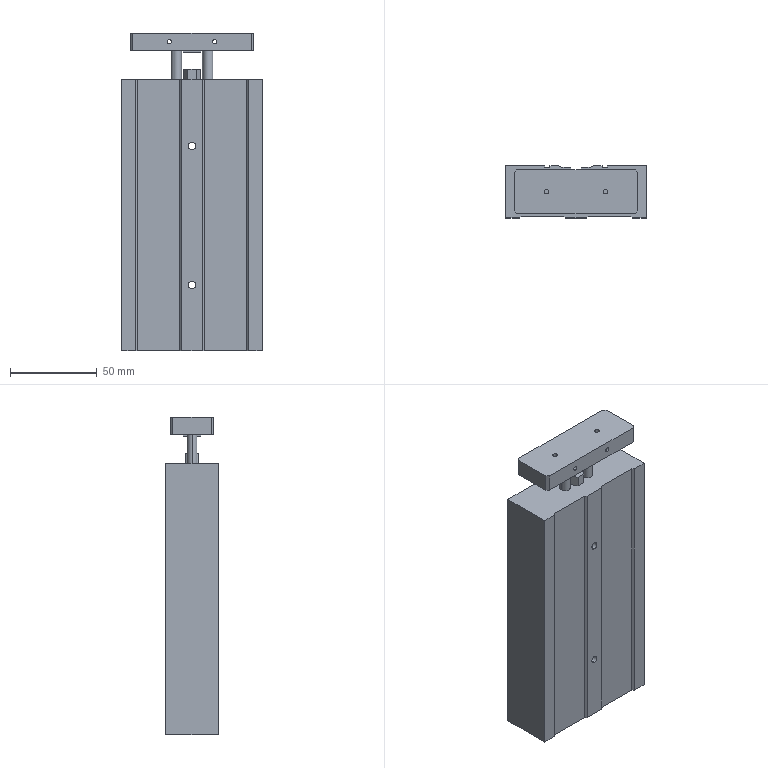Part | SolidWorks | features Boss 4, HoleWzd 3, Extrusion 1 | 2 solids | 73 faces | box 81 x 30 x 183 mm | volume 382969 mm3 | plane 57 | cylinder 16 | commonest cylinder face diameters 2.5 x8 4.2 x4 6 x4